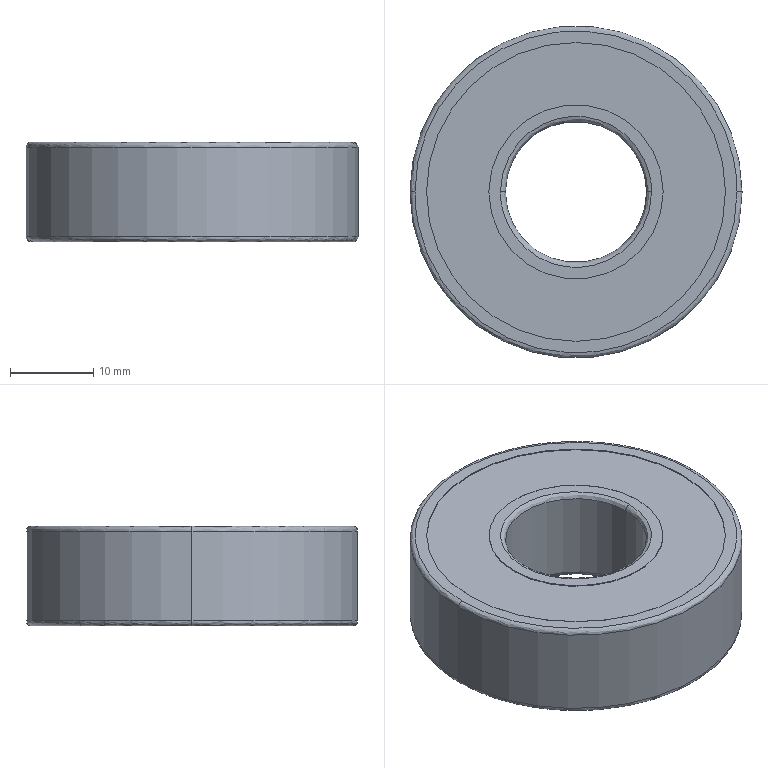Part | SolidWorks | features BaseBody 1 | 1 solid | 26 faces | box 40 x 40 x 12 mm | volume 12195 mm3 | cylinder 12 | spline 8 | plane 6 | commonest cylinder face diameters 21 x4 36 x4 17 x2 40 x2
STEP:
#1=CARTESIAN_POINT('',(-19.4,0.,-12.));
#2=VERTEX_POINT('',#1);
#3=CARTESIAN_POINT('',(19.4,0.,-12.));
#4=VERTEX_POINT('',#3);
#5=CARTESIAN_POINT('',(-19.4,0.,-12.));
#6=CARTESIAN_POINT('',(-19.4,-38.8,-12.));
#7=CARTESIAN_POINT('',(19.4,-38.8,-12.));
#8=CARTESIAN_POINT('',(19.4,0.,-12.));
#9=(BOUNDED_CURVE()B_SPLINE_CURVE(3,(#5,#6,#7,#8),.UNSPECIFIED.,.F.,.F.)B_SPLINE_CURVE_WITH_KNOTS((4,4),(0.,0.5),.UNSPECIFIED.)CURVE()GEOMETRIC_REPRESENTATION_ITEM()RATIONAL_B_SPLINE_CURVE((1.,0.3333,0.3333,1.))REPRESENTATION_ITEM(''));
#10=EDGE_CURVE('',#2,#4,#9,.T.);
#11=ORIENTED_EDGE('',*,*,#10,.T.);
#12=CARTESIAN_POINT('',(20.,0.,-11.4));
#13=VERTEX_POINT('',#12);
#14=CARTESIAN_POINT('',(19.4,0.,-11.4));
#15=DIRECTION('',(0.,-1.,0.));
#16=DIRECTION('',(1.,0.,0.));
#17=AXIS2_PLACEMENT_3D('',#14,#15,#16);
#18=CIRCLE('',#17,0.6);
#19=EDGE_CURVE('',#4,#13,#18,.T.);
#20=ORIENTED_EDGE('',*,*,#19,.T.);
#21=CARTESIAN_POINT('',(-20.,0.,-11.4));
#22=VERTEX_POINT('',#21);
#23=CARTESIAN_POINT('',(0.,0.,-11.4));
#24=DIRECTION('',(0.,0.,1.));
#25=DIRECTION('',(1.,0.,0.));
#26=AXIS2_PLACEMENT_3D('',#23,#24,#25);
#27=CIRCLE('',#26,20.);
#28=EDGE_CURVE('',#22,#13,#27,.T.);
#29=ORIENTED_EDGE('',*,*,#28,.F.);
#30=CARTESIAN_POINT('',(-19.4,0.,-11.4));
#31=DIRECTION('',(0.,1.,0.));
#32=DIRECTION('',(-1.,0.,0.));
#33=AXIS2_PLACEMENT_3D('',#30,#31,#32);
#34=CIRCLE('',#33,0.6);
#35=EDGE_CURVE('',#2,#22,#34,.T.);
#36=ORIENTED_EDGE('',*,*,#35,.F.);
#37=EDGE_LOOP('',(#11,#20,#29,#36));
#38=FACE_OUTER_BOUND('',#37,.T.);
#39=CARTESIAN_POINT('',(19.4,0.,-12.));
#40=CARTESIAN_POINT('',(19.4,-38.8,-12.));
#41=CARTESIAN_POINT('',(-19.4,-38.8,-12.));
#42=CARTESIAN_POINT('',(-19.4,0.,-12.));
#43=CARTESIAN_POINT('',(19.751,0.,-12.));
#44=CARTESIAN_POINT('',(19.751,-39.503,-12.));
#45=CARTESIAN_POINT('',(-19.751,-39.503,-12.));
#46=CARTESIAN_POINT('',(-19.751,0.,-12.));
#47=CARTESIAN_POINT('',(20.,0.,-11.751));
#48=CARTESIAN_POINT('',(20.,-40.,-11.751));
#49=CARTESIAN_POINT('',(-20.,-40.,-11.751));
#50=CARTESIAN_POINT('',(-20.,0.,-11.751));
#51=CARTESIAN_POINT('',(20.,0.,-11.4));
#52=CARTESIAN_POINT('',(20.,-40.,-11.4));
#53=CARTESIAN_POINT('',(-20.,-40.,-11.4));
#54=CARTESIAN_POINT('',(-20.,0.,-11.4));
#55=(BOUNDED_SURFACE()B_SPLINE_SURFACE(3,3,((#39,#40,#41,#42),(#43,#44,#45,#46),(#47,#48,#49,#50),(#51,#52,#53,#54)),.UNSPECIFIED.,.F.,.F.,.F.)B_SPLINE_SURFACE_WITH_KNOTS((4,4),(4,4),(0.,1.),(0.,1.),.UNSPECIFIED.)GEOMETRIC_REPRESENTATION_ITEM()RATIONAL_B_SPLINE_SURFACE(((1.,0.3333,0.3333,1.),(0.8047,0.2682,0.2682,0.8047),(0.8047,0.2682,0.2682,0.8047),(1.,0.3333,0.3333,1.)))REPRESENTATION_ITEM('')SURFACE());
#56=ADVANCED_FACE('',(#38),#55,.T.);
#57=CARTESIAN_POINT('',(20.,0.,-0.6));
#58=VERTEX_POINT('',#57);
#59=CARTESIAN_POINT('',(-20.,0.,-0.6));
#60=VERTEX_POINT('',#59);
#61=CARTESIAN_POINT('',(0.,0.,-0.6));
#62=DIRECTION('',(0.,0.,-1.));
#63=DIRECTION('',(1.,0.,0.));
#64=AXIS2_PLACEMENT_3D('',#61,#62,#63);
#65=CIRCLE('',#64,20.);
#66=EDGE_CURVE('',#58,#60,#65,.T.);
#67=ORIENTED_EDGE('',*,*,#66,.F.);
#68=CARTESIAN_POINT('',(19.4,0.,0.));
#69=VERTEX_POINT('',#68);
#70=CARTESIAN_POINT('',(19.4,0.,-0.6));
#71=DIRECTION('',(0.,-1.,0.));
#72=DIRECTION('',(1.,0.,0.));
#73=AXIS2_PLACEMENT_3D('',#70,#71,#72);
#74=CIRCLE('',#73,0.6);
#75=EDGE_CURVE('',#58,#69,#74,.T.);
#76=ORIENTED_EDGE('',*,*,#75,.T.);
#77=CARTESIAN_POINT('',(-19.4,0.,0.));
#78=VERTEX_POINT('',#77);
#79=CARTESIAN_POINT('',(19.4,0.,0.));
#80=CARTESIAN_POINT('',(19.4,-38.8,0.));
#81=CARTESIAN_POINT('',(-19.4,-38.8,0.));
#82=CARTESIAN_POINT('',(-19.4,0.,0.));
#83=(BOUNDED_CURVE()B_SPLINE_CURVE(3,(#79,#80,#81,#82),.UNSPECIFIED.,.F.,.F.)B_SPLINE_CURVE_WITH_KNOTS((4,4),(0.5,1.),.UNSPECIFIED.)CURVE()GEOMETRIC_REPRESENTATION_ITEM()RATIONAL_B_SPLINE_CURVE((1.,0.3333,0.3333,1.))REPRESENTATION_ITEM(''));
#84=EDGE_CURVE('',#69,#78,#83,.T.);
#85=ORIENTED_EDGE('',*,*,#84,.T.);
#86=CARTESIAN_POINT('',(-19.4,0.,-0.6));
#87=DIRECTION('',(0.,1.,0.));
#88=DIRECTION('',(-1.,0.,0.));
#89=AXIS2_PLACEMENT_3D('',#86,#87,#88);
#90=CIRCLE('',#89,0.6);
#91=EDGE_CURVE('',#60,#78,#90,.T.);
#92=ORIENTED_EDGE('',*,*,#91,.F.);
#93=EDGE_LOOP('',(#67,#76,#85,#92));
#94=FACE_OUTER_BOUND('',#93,.T.);
#95=CARTESIAN_POINT('',(20.,0.,-0.6));
#96=CARTESIAN_POINT('',(20.,-40.,-0.6));
#97=CARTESIAN_POINT('',(-20.,-40.,-0.6));
#98=CARTESIAN_POINT('',(-20.,0.,-0.6));
#99=CARTESIAN_POINT('',(20.,0.,-0.2485));
#100=CARTESIAN_POINT('',(20.,-40.,-0.2485));
#101=CARTESIAN_POINT('',(-20.,-40.,-0.2485));
#102=CARTESIAN_POINT('',(-20.,0.,-0.2485));
#103=CARTESIAN_POINT('',(19.751,0.,0.));
#104=CARTESIAN_POINT('',(19.751,-39.503,0.));
#105=CARTESIAN_POINT('',(-19.751,-39.503,0.));
#106=CARTESIAN_POINT('',(-19.751,0.,0.));
#107=CARTESIAN_POINT('',(19.4,0.,0.));
#108=CARTESIAN_POINT('',(19.4,-38.8,0.));
#109=CARTESIAN_POINT('',(-19.4,-38.8,0.));
#110=CARTESIAN_POINT('',(-19.4,0.,0.));
#111=(BOUNDED_SURFACE()B_SPLINE_SURFACE(3,3,((#95,#96,#97,#98),(#99,#100,#101,#102),(#103,#104,#105,#106),(#107,#108,#109,#110)),.UNSPECIFIED.,.F.,.F.,.F.)B_SPLINE_SURFACE_WITH_KNOTS((4,4),(4,4),(0.,1.),(0.,1.),.UNSPECIFIED.)GEOMETRIC_REPRESENTATION_ITEM()RATIONAL_B_SPLINE_SURFACE(((1.,0.3333,0.3333,1.),(0.8047,0.2682,0.2682,0.8047),(0.8047,0.2682,0.2682,0.8047),(1.,0.3333,0.3333,1.)))REPRESENTATION_ITEM('')SURFACE());
#112=ADVANCED_FACE('',(#94),#111,.T.);
#113=CARTESIAN_POINT('',(-8.5,0.,-11.4));
#114=VERTEX_POINT('',#113);
#115=CARTESIAN_POINT('',(8.5,0.,-11.4));
#116=VERTEX_POINT('',#115);
#117=CARTESIAN_POINT('',(0.,0.,-11.4));
#118=DIRECTION('',(0.,0.,1.));
#119=DIRECTION('',(-1.,0.,0.));
#120=AXIS2_PLACEMENT_3D('',#117,#118,#119);
#121=CIRCLE('',#120,8.5);
#122=EDGE_CURVE('',#114,#116,#121,.T.);
#123=ORIENTED_EDGE('',*,*,#122,.T.);
#124=CARTESIAN_POINT('',(9.1,0.,-12.));
#125=VERTEX_POINT('',#124);
#126=CARTESIAN_POINT('',(9.1,0.,-11.4));
#127=DIRECTION('',(0.,-1.,0.));
#128=DIRECTION('',(1.,0.,0.));
#129=AXIS2_PLACEMENT_3D('',#126,#127,#128);
#130=CIRCLE('',#129,0.6);
#131=EDGE_CURVE('',#116,#125,#130,.T.);
#132=ORIENTED_EDGE('',*,*,#131,.T.);
#133=CARTESIAN_POINT('',(-9.1,0.,-12.));
#134=VERTEX_POINT('',#133);
#135=CARTESIAN_POINT('',(-9.1,0.,-12.));
#136=CARTESIAN_POINT('',(-9.1,-0.2782,-12.));
#137=CARTESIAN_POINT('',(-9.081,-0.6939,-12.));
#138=CARTESIAN_POINT('',(-9.026,-1.176,-12.));
#139=CARTESIAN_POINT('',(-8.99,-1.416,-12.));
#140=CARTESIAN_POINT('',(-8.972,-1.519,-12.));
#141=CARTESIAN_POINT('',(-8.961,-1.587,-12.));
#142=CARTESIAN_POINT('',(-8.955,-1.62,-12.));
#143=CARTESIAN_POINT('',(-8.894,-1.946,-12.));
#144=CARTESIAN_POINT('',(-8.793,-2.375,-12.));
#145=CARTESIAN_POINT('',(-8.639,-2.866,-12.));
#146=CARTESIAN_POINT('',(-8.553,-3.109,-12.));
#147=CARTESIAN_POINT('',(-8.514,-3.212,-12.));
#148=CARTESIAN_POINT('',(-8.488,-3.281,-12.));
#149=CARTESIAN_POINT('',(-8.475,-3.314,-12.));
#150=CARTESIAN_POINT('',(-8.348,-3.635,-12.));
#151=CARTESIAN_POINT('',(-8.158,-4.054,-12.));
#152=CARTESIAN_POINT('',(-7.899,-4.523,-12.));
#153=CARTESIAN_POINT('',(-7.781,-4.72,-12.));
#154=CARTESIAN_POINT('',(-7.7,-4.85,-12.));
#155=CARTESIAN_POINT('',(-7.66,-4.914,-12.));
#156=CARTESIAN_POINT('',(-7.273,-5.505,-12.));
#157=CARTESIAN_POINT('',(-6.879,-5.991,-12.));
#158=CARTESIAN_POINT('',(-6.213,-6.657,-12.));
#159=CARTESIAN_POINT('',(-5.864,-6.971,-12.));
#160=CARTESIAN_POINT('',(-5.431,-7.305,-12.));
#161=CARTESIAN_POINT('',(-5.239,-7.441,-12.));
#162=CARTESIAN_POINT('',(-5.11,-7.53,-12.));
#163=CARTESIAN_POINT('',(-5.044,-7.575,-12.));
#164=CARTESIAN_POINT('',(-4.722,-7.785,-12.));
#165=CARTESIAN_POINT('',(-4.326,-8.017,-12.));
#166=CARTESIAN_POINT('',(-3.844,-8.251,-12.));
#167=CARTESIAN_POINT('',(-3.598,-8.359,-12.));
#168=CARTESIAN_POINT('',(-3.492,-8.403,-12.));
#169=CARTESIAN_POINT('',(-3.421,-8.433,-12.));
#170=CARTESIAN_POINT('',(-3.384,-8.448,-12.));
#171=CARTESIAN_POINT('',(-3.075,-8.57,-12.));
#172=CARTESIAN_POINT('',(-2.658,-8.712,-12.));
#173=CARTESIAN_POINT('',(-2.16,-8.842,-12.));
#174=CARTESIAN_POINT('',(-1.909,-8.898,-12.));
#175=CARTESIAN_POINT('',(-1.801,-8.92,-12.));
#176=CARTESIAN_POINT('',(-1.728,-8.934,-12.));
#177=CARTESIAN_POINT('',(-1.69,-8.942,-12.));
#178=CARTESIAN_POINT('',(-1.109,-9.049,-12.));
#179=CARTESIAN_POINT('',(-0.5562,-9.1,-12.));
#180=CARTESIAN_POINT('',(0.2781,-9.1,-12.));
#181=CARTESIAN_POINT('',(0.6937,-9.081,-12.));
#182=CARTESIAN_POINT('',(1.176,-9.026,-12.));
#183=CARTESIAN_POINT('',(1.416,-8.99,-12.));
#184=CARTESIAN_POINT('',(1.519,-8.972,-12.));
#185=CARTESIAN_POINT('',(1.587,-8.961,-12.));
#186=CARTESIAN_POINT('',(1.62,-8.955,-12.));
#187=CARTESIAN_POINT('',(1.946,-8.894,-12.));
#188=CARTESIAN_POINT('',(2.375,-8.793,-12.));
#189=CARTESIAN_POINT('',(2.866,-8.639,-12.));
#190=CARTESIAN_POINT('',(3.109,-8.553,-12.));
#191=CARTESIAN_POINT('',(3.212,-8.514,-12.));
#192=CARTESIAN_POINT('',(3.281,-8.488,-12.));
#193=CARTESIAN_POINT('',(3.314,-8.475,-12.));
#194=CARTESIAN_POINT('',(3.635,-8.348,-12.));
#195=CARTESIAN_POINT('',(4.054,-8.158,-12.));
#196=CARTESIAN_POINT('',(4.523,-7.899,-12.));
#197=CARTESIAN_POINT('',(4.72,-7.781,-12.));
#198=CARTESIAN_POINT('',(4.85,-7.7,-12.));
#199=CARTESIAN_POINT('',(4.914,-7.66,-12.));
#200=CARTESIAN_POINT('',(5.505,-7.273,-12.));
#201=CARTESIAN_POINT('',(5.991,-6.879,-12.));
#202=CARTESIAN_POINT('',(6.657,-6.213,-12.));
#203=CARTESIAN_POINT('',(6.971,-5.864,-12.));
#204=CARTESIAN_POINT('',(7.305,-5.431,-12.));
#205=CARTESIAN_POINT('',(7.441,-5.239,-12.));
#206=CARTESIAN_POINT('',(7.53,-5.11,-12.));
#207=CARTESIAN_POINT('',(7.575,-5.044,-12.));
#208=CARTESIAN_POINT('',(7.785,-4.722,-12.));
#209=CARTESIAN_POINT('',(8.017,-4.326,-12.));
#210=CARTESIAN_POINT('',(8.251,-3.844,-12.));
#211=CARTESIAN_POINT('',(8.359,-3.598,-12.));
#212=CARTESIAN_POINT('',(8.403,-3.492,-12.));
#213=CARTESIAN_POINT('',(8.433,-3.421,-12.));
#214=CARTESIAN_POINT('',(8.448,-3.384,-12.));
#215=CARTESIAN_POINT('',(8.57,-3.075,-12.));
#216=CARTESIAN_POINT('',(8.712,-2.658,-12.));
#217=CARTESIAN_POINT('',(8.842,-2.16,-12.));
#218=CARTESIAN_POINT('',(8.898,-1.909,-12.));
#219=CARTESIAN_POINT('',(8.92,-1.801,-12.));
#220=CARTESIAN_POINT('',(8.934,-1.728,-12.));
#221=CARTESIAN_POINT('',(8.942,-1.69,-12.));
#222=CARTESIAN_POINT('',(9.049,-1.109,-12.));
#223=CARTESIAN_POINT('',(9.1,-0.5562,-12.));
#224=CARTESIAN_POINT('',(9.1,0.,-12.));
#225=B_SPLINE_CURVE_WITH_KNOTS('',3,(#135,#136,#137,#138,#139,#140,#141,#142,#143,#144,#145,#146,#147,#148,#149,#150,#151,#152,#153,#154,#155,#156,#157,#158,#159,#160,#161,#162,#163,#164,#165,#166,#167,#168,#169,#170,#171,#172,#173,#174,#175,#176,#177,#178,#179,#180,#181,#182,#183,#184,#185,#186,#187,#188,#189,#190,#191,#192,#193,#194,#195,#196,#197,#198,#199,#200,#201,#202,#203,#204,#205,#206,#207,#208,#209,#210,#211,#212,#213,#214,#215,#216,#217,#218,#219,#220,#221,#222,#223,#224),.UNSPECIFIED.,.F.,.F.,(4,1,1,1,2,2,1,1,1,2,2,1,1,2,2,2,1,1,2,2,1,1,1,2,2,1,1,1,2,2,2,1,1,1,2,2,1,1,1,2,2,1,1,2,2,2,1,1,2,2,1,1,1,2,2,1,1,1,2,2,4),(0.,0.01562,0.02344,0.02734,0.0293,0.03125,0.04687,0.05469,0.05859,0.06055,0.0625,0.07812,0.08594,0.08984,0.09375,0.125,0.1406,0.1484,0.1523,0.1562,0.1719,0.1797,0.1836,0.1855,0.1875,0.2031,0.2109,0.2148,0.2168,0.2187,0.25,0.2656,0.2734,0.2773,0.2793,0.2812,0.2969,0.3047,0.3086,0.3105,0.3125,0.3281,0.3359,0.3398,0.3437,0.375,0.3906,0.3984,0.4023,0.4062,0.4219,0.4297,0.4336,0.4355,0.4375,0.4531,0.4609,0.4648,0.4668,0.4687,0.5),.UNSPECIFIED.);
#226=EDGE_CURVE('',#134,#125,#225,.T.);
#227=ORIENTED_EDGE('',*,*,#226,.F.);
#228=CARTESIAN_POINT('',(-9.1,0.,-11.4));
#229=DIRECTION('',(0.,1.,0.));
#230=DIRECTION('',(-1.,0.,0.));
#231=AXIS2_PLACEMENT_3D('',#228,#229,#230);
#232=CIRCLE('',#231,0.6);
#233=EDGE_CURVE('',#114,#134,#232,.T.);
#234=ORIENTED_EDGE('',*,*,#233,.F.);
#235=EDGE_LOOP('',(#123,#132,#227,#234));
#236=FACE_OUTER_BOUND('',#235,.T.);
#237=CARTESIAN_POINT('',(8.5,0.,-11.4));
#238=CARTESIAN_POINT('',(8.5,-17.,-11.4));
#239=CARTESIAN_POINT('',(-8.5,-17.,-11.4));
#240=CARTESIAN_POINT('',(-8.5,0.,-11.4));
#241=CARTESIAN_POINT('',(8.5,0.,-11.751));
#242=CARTESIAN_POINT('',(8.5,-17.,-11.751));
#243=CARTESIAN_POINT('',(-8.5,-17.,-11.751));
#244=CARTESIAN_POINT('',(-8.5,0.,-11.751));
#245=CARTESIAN_POINT('',(8.749,0.,-12.));
#246=CARTESIAN_POINT('',(8.749,-17.497,-12.));
#247=CARTESIAN_POINT('',(-8.749,-17.497,-12.));
#248=CARTESIAN_POINT('',(-8.749,0.,-12.));
#249=CARTESIAN_POINT('',(9.1,0.,-12.));
#250=CARTESIAN_POINT('',(9.1,-18.2,-12.));
#251=CARTESIAN_POINT('',(-9.1,-18.2,-12.));
#252=CARTESIAN_POINT('',(-9.1,0.,-12.));
#253=(BOUNDED_SURFACE()B_SPLINE_SURFACE(3,3,((#237,#238,#239,#240),(#241,#242,#243,#244),(#245,#246,#247,#248),(#249,#250,#251,#252)),.UNSPECIFIED.,.F.,.F.,.F.)B_SPLINE_SURFACE_WITH_KNOTS((4,4),(4,4),(0.,1.),(0.,1.),.UNSPECIFIED.)GEOMETRIC_REPRESENTATION_ITEM()RATIONAL_B_SPLINE_SURFACE(((1.,0.3333,0.3333,1.),(0.8047,0.2682,0.2682,0.8047),(0.8047,0.2682,0.2682,0.8047),(1.,0.3333,0.3333,1.)))REPRESENTATION_ITEM('')SURFACE());
#254=ADVANCED_FACE('',(#236),#253,.T.);
#255=CARTESIAN_POINT('',(9.1,0.,0.));
#256=VERTEX_POINT('',#255);
#257=CARTESIAN_POINT('',(-9.1,0.,0.));
#258=VERTEX_POINT('',#257);
#259=CARTESIAN_POINT('',(9.1,0.,0.));
#260=CARTESIAN_POINT('',(9.1,-0.2781,0.));
#261=CARTESIAN_POINT('',(9.081,-0.6937,0.));
#262=CARTESIAN_POINT('',(9.026,-1.176,0.));
#263=CARTESIAN_POINT('',(8.99,-1.416,0.));
#264=CARTESIAN_POINT('',(8.972,-1.519,0.));
#265=CARTESIAN_POINT('',(8.961,-1.587,0.));
#266=CARTESIAN_POINT('',(8.955,-1.62,0.));
#267=CARTESIAN_POINT('',(8.894,-1.946,0.));
#268=CARTESIAN_POINT('',(8.793,-2.375,0.));
#269=CARTESIAN_POINT('',(8.639,-2.866,0.));
#270=CARTESIAN_POINT('',(8.553,-3.109,0.));
#271=CARTESIAN_POINT('',(8.514,-3.212,0.));
#272=CARTESIAN_POINT('',(8.488,-3.281,0.));
#273=CARTESIAN_POINT('',(8.475,-3.314,0.));
#274=CARTESIAN_POINT('',(8.348,-3.635,0.));
#275=CARTESIAN_POINT('',(8.158,-4.054,0.));
#276=CARTESIAN_POINT('',(7.899,-4.523,0.));
#277=CARTESIAN_POINT('',(7.781,-4.72,0.));
#278=CARTESIAN_POINT('',(7.7,-4.85,0.));
#279=CARTESIAN_POINT('',(7.66,-4.914,0.));
#280=CARTESIAN_POINT('',(7.273,-5.505,0.));
#281=CARTESIAN_POINT('',(6.879,-5.991,0.));
#282=CARTESIAN_POINT('',(6.213,-6.657,0.));
#283=CARTESIAN_POINT('',(5.864,-6.971,0.));
#284=CARTESIAN_POINT('',(5.431,-7.305,0.));
#285=CARTESIAN_POINT('',(5.239,-7.441,0.));
#286=CARTESIAN_POINT('',(5.11,-7.53,0.));
#287=CARTESIAN_POINT('',(5.044,-7.575,0.));
#288=CARTESIAN_POINT('',(4.722,-7.785,0.));
#289=CARTESIAN_POINT('',(4.326,-8.017,0.));
#290=CARTESIAN_POINT('',(3.844,-8.251,0.));
#291=CARTESIAN_POINT('',(3.598,-8.359,0.));
#292=CARTESIAN_POINT('',(3.492,-8.403,0.));
#293=CARTESIAN_POINT('',(3.421,-8.433,0.));
#294=CARTESIAN_POINT('',(3.384,-8.448,0.));
#295=CARTESIAN_POINT('',(3.075,-8.57,0.));
#296=CARTESIAN_POINT('',(2.658,-8.712,0.));
#297=CARTESIAN_POINT('',(2.16,-8.842,0.));
#298=CARTESIAN_POINT('',(1.909,-8.898,0.));
#299=CARTESIAN_POINT('',(1.801,-8.92,0.));
#300=CARTESIAN_POINT('',(1.728,-8.934,0.));
#301=CARTESIAN_POINT('',(1.69,-8.942,0.));
#302=CARTESIAN_POINT('',(1.109,-9.049,0.));
#303=CARTESIAN_POINT('',(0.5562,-9.1,0.));
#304=CARTESIAN_POINT('',(-0.2781,-9.1,0.));
#305=CARTESIAN_POINT('',(-0.6937,-9.081,0.));
#306=CARTESIAN_POINT('',(-1.176,-9.026,0.));
#307=CARTESIAN_POINT('',(-1.416,-8.99,0.));
#308=CARTESIAN_POINT('',(-1.519,-8.972,0.));
#309=CARTESIAN_POINT('',(-1.587,-8.961,0.));
#310=CARTESIAN_POINT('',(-1.62,-8.955,0.));
#311=CARTESIAN_POINT('',(-1.946,-8.894,0.));
#312=CARTESIAN_POINT('',(-2.375,-8.793,0.));
#313=CARTESIAN_POINT('',(-2.866,-8.639,0.));
#314=CARTESIAN_POINT('',(-3.109,-8.553,0.));
#315=CARTESIAN_POINT('',(-3.212,-8.514,0.));
#316=CARTESIAN_POINT('',(-3.281,-8.488,0.));
#317=CARTESIAN_POINT('',(-3.314,-8.475,0.));
#318=CARTESIAN_POINT('',(-3.635,-8.348,0.));
#319=CARTESIAN_POINT('',(-4.054,-8.158,0.));
#320=CARTESIAN_POINT('',(-4.523,-7.899,0.));
#321=CARTESIAN_POINT('',(-4.72,-7.781,0.));
#322=CARTESIAN_POINT('',(-4.85,-7.7,0.));
#323=CARTESIAN_POINT('',(-4.914,-7.66,0.));
#324=CARTESIAN_POINT('',(-5.505,-7.273,0.));
#325=CARTESIAN_POINT('',(-5.991,-6.879,0.));
#326=CARTESIAN_POINT('',(-6.657,-6.213,0.));
#327=CARTESIAN_POINT('',(-6.971,-5.864,0.));
#328=CARTESIAN_POINT('',(-7.305,-5.431,0.));
#329=CARTESIAN_POINT('',(-7.441,-5.239,0.));
#330=CARTESIAN_POINT('',(-7.53,-5.11,0.));
#331=CARTESIAN_POINT('',(-7.575,-5.044,0.));
#332=CARTESIAN_POINT('',(-7.785,-4.722,0.));
#333=CARTESIAN_POINT('',(-8.017,-4.326,0.));
#334=CARTESIAN_POINT('',(-8.251,-3.844,0.));
#335=CARTESIAN_POINT('',(-8.359,-3.598,0.));
#336=CARTESIAN_POINT('',(-8.403,-3.492,0.));
#337=CARTESIAN_POINT('',(-8.433,-3.421,0.));
#338=CARTESIAN_POINT('',(-8.448,-3.384,0.));
#339=CARTESIAN_POINT('',(-8.57,-3.075,0.));
#340=CARTESIAN_POINT('',(-8.712,-2.658,0.));
#341=CARTESIAN_POINT('',(-8.842,-2.16,0.));
#342=CARTESIAN_POINT('',(-8.898,-1.909,0.));
#343=CARTESIAN_POINT('',(-8.92,-1.801,0.));
#344=CARTESIAN_POINT('',(-8.934,-1.728,0.));
#345=CARTESIAN_POINT('',(-8.942,-1.69,0.));
#346=CARTESIAN_POINT('',(-9.049,-1.109,0.));
#347=CARTESIAN_POINT('',(-9.1,-0.5568,0.));
#348=CARTESIAN_POINT('',(-9.1,0.,0.));
#349=B_SPLINE_CURVE_WITH_KNOTS('',3,(#259,#260,#261,#262,#263,#264,#265,#266,#267,#268,#269,#270,#271,#272,#273,#274,#275,#276,#277,#278,#279,#280,#281,#282,#283,#284,#285,#286,#287,#288,#289,#290,#291,#292,#293,#294,#295,#296,#297,#298,#299,#300,#301,#302,#303,#304,#305,#306,#307,#308,#309,#310,#311,#312,#313,#314,#315,#316,#317,#318,#319,#320,#321,#322,#323,#324,#325,#326,#327,#328,#329,#330,#331,#332,#333,#334,#335,#336,#337,#338,#339,#340,#341,#342,#343,#344,#345,#346,#347,#348),.UNSPECIFIED.,.F.,.F.,(4,1,1,1,2,2,1,1,1,2,2,1,1,2,2,2,1,1,2,2,1,1,1,2,2,1,1,1,2,2,2,1,1,1,2,2,1,1,1,2,2,1,1,2,2,2,1,1,2,2,1,1,1,2,2,1,1,1,2,2,4),(0.5,0.5156,0.5234,0.5273,0.5293,0.5312,0.5469,0.5547,0.5586,0.5605,0.5625,0.5781,0.5859,0.5898,0.5937,0.625,0.6406,0.6484,0.6523,0.6562,0.6719,0.6797,0.6836,0.6855,0.6875,0.7031,0.7109,0.7148,0.7168,0.7188,0.75,0.7656,0.7734,0.7773,0.7793,0.7812,0.7969,0.8047,0.8086,0.8105,0.8125,0.8281,0.8359,0.8398,0.8437,0.875,0.8906,0.8984,0.9023,0.9062,0.9219,0.9297,0.9336,0.9355,0.9375,0.9531,0.9609,0.9648,0.9668,0.9687,1.),.UNSPECIFIED.);
#350=EDGE_CURVE('',#256,#258,#349,.T.);
#351=ORIENTED_EDGE('',*,*,#350,.F.);
#352=CARTESIAN_POINT('',(8.5,0.,-0.6));
#353=VERTEX_POINT('',#352);
#354=CARTESIAN_POINT('',(9.1,0.,-0.6));
#355=DIRECTION('',(0.,-1.,0.));
#356=DIRECTION('',(1.,0.,0.));
#357=AXIS2_PLACEMENT_3D('',#354,#355,#356);
#358=CIRCLE('',#357,0.6);
#359=EDGE_CURVE('',#256,#353,#358,.T.);
#360=ORIENTED_EDGE('',*,*,#359,.T.);
#361=CARTESIAN_POINT('',(-8.5,0.,-0.6));
#362=VERTEX_POINT('',#361);
#363=CARTESIAN_POINT('',(0.,0.,-0.6));
#364=DIRECTION('',(0.,0.,-1.));
#365=DIRECTION('',(-1.,0.,0.));
#366=AXIS2_PLACEMENT_3D('',#363,#364,#365);
#367=CIRCLE('',#366,8.5);
#368=EDGE_CURVE('',#353,#362,#367,.T.);
#369=ORIENTED_EDGE('',*,*,#368,.T.);
#370=CARTESIAN_POINT('',(-9.1,0.,-0.6));
#371=DIRECTION('',(0.,1.,0.));
#372=DIRECTION('',(-1.,0.,0.));
#373=AXIS2_PLACEMENT_3D('',#370,#371,#372);
#374=CIRCLE('',#373,0.6);
#375=EDGE_CURVE('',#258,#362,#374,.T.);
#376=ORIENTED_EDGE('',*,*,#375,.F.);
#377=EDGE_LOOP('',(#351,#360,#369,#376));
#378=FACE_OUTER_BOUND('',#377,.T.);
#379=CARTESIAN_POINT('',(9.1,0.,0.));
#380=CARTESIAN_POINT('',(9.1,-18.2,0.));
#381=CARTESIAN_POINT('',(-9.1,-18.2,0.));
#382=CARTESIAN_POINT('',(-9.1,0.,0.));
#383=CARTESIAN_POINT('',(8.749,0.,0.));
#384=CARTESIAN_POINT('',(8.749,-17.497,0.));
#385=CARTESIAN_POINT('',(-8.749,-17.497,0.));
#386=CARTESIAN_POINT('',(-8.749,0.,0.));
#387=CARTESIAN_POINT('',(8.5,0.,-0.2485));
#388=CARTESIAN_POINT('',(8.5,-17.,-0.2485));
#389=CARTESIAN_POINT('',(-8.5,-17.,-0.2485));
#390=CARTESIAN_POINT('',(-8.5,0.,-0.2485));
#391=CARTESIAN_POINT('',(8.5,0.,-0.6));
#392=CARTESIAN_POINT('',(8.5,-17.,-0.6));
#393=CARTESIAN_POINT('',(-8.5,-17.,-0.6));
#394=CARTESIAN_POINT('',(-8.5,0.,-0.6));
#395=(BOUNDED_SURFACE()B_SPLINE_SURFACE(3,3,((#379,#380,#381,#382),(#383,#384,#385,#386),(#387,#388,#389,#390),(#391,#392,#393,#394)),.UNSPECIFIED.,.F.,.F.,.F.)B_SPLINE_SURFACE_WITH_KNOTS((4,4),(4,4),(0.,1.),(0.,1.),.UNSPECIFIED.)GEOMETRIC_REPRESENTATION_ITEM()RATIONAL_B_SPLINE_SURFACE(((1.,0.3333,0.3333,1.),(0.8047,0.2682,0.2682,0.8047),(0.8047,0.2682,0.2682,0.8047),(1.,0.3333,0.3333,1.)))REPRESENTATION_ITEM('')SURFACE());
#396=ADVANCED_FACE('',(#378),#395,.T.);
#397=CARTESIAN_POINT('',(0.,0.,-11.4));
#398=DIRECTION('',(0.,0.,1.));
#399=DIRECTION('',(1.,0.,0.));
#400=AXIS2_PLACEMENT_3D('',#397,#398,#399);
#401=CIRCLE('',#400,20.);
#402=EDGE_CURVE('',#13,#22,#401,.T.);
#403=ORIENTED_EDGE('',*,*,#402,.T.);
#404=CARTESIAN_POINT('',(-20.,0.,-12.));
#405=DIRECTION('',(0.,0.,1.));
#406=VECTOR('',#405,1000.);
#407=LINE('',#404,#406);
#408=EDGE_CURVE('',#22,#60,#407,.T.);
#409=ORIENTED_EDGE('',*,*,#408,.T.);
#410=CARTESIAN_POINT('',(0.,0.,-0.6));
#411=DIRECTION('',(0.,0.,-1.));
#412=DIRECTION('',(1.,0.,0.));
#413=AXIS2_PLACEMENT_3D('',#410,#411,#412);
#414=CIRCLE('',#413,20.);
#415=EDGE_CURVE('',#60,#58,#414,.T.);
#416=ORIENTED_EDGE('',*,*,#415,.T.);
#417=CARTESIAN_POINT('',(20.,0.,-12.));
#418=DIRECTION('',(0.,0.,1.));
#419=VECTOR('',#418,1000.);
#420=LINE('',#417,#419);
#421=EDGE_CURVE('',#13,#58,#420,.T.);
#422=ORIENTED_EDGE('',*,*,#421,.F.);
#423=EDGE_LOOP('',(#403,#409,#416,#422));
#424=FACE_OUTER_BOUND('',#423,.T.);
#425=CARTESIAN_POINT('',(0.,0.,-12.));
#426=DIRECTION('',(0.,0.,1.));
#427=DIRECTION('',(1.,0.,0.));
#428=AXIS2_PLACEMENT_3D('',#425,#426,#427);
#429=CYLINDRICAL_SURFACE('',#428,20.);
#430=ADVANCED_FACE('',(#424),#429,.T.);
#431=CARTESIAN_POINT('',(-18.,0.,-12.));
#432=VERTEX_POINT('',#431);
#433=CARTESIAN_POINT('',(18.,0.,-12.));
#434=VERTEX_POINT('',#433);
#435=CARTESIAN_POINT('',(0.,0.,-12.));
#436=DIRECTION('',(0.,0.,1.));
#437=DIRECTION('',(1.,0.,0.));
#438=AXIS2_PLACEMENT_3D('',#435,#436,#437);
#439=CIRCLE('',#438,18.);
#440=EDGE_CURVE('',#432,#434,#439,.T.);
#441=ORIENTED_EDGE('',*,*,#440,.F.);
#442=CARTESIAN_POINT('',(-18.,0.,-11.9));
#443=VERTEX_POINT('',#442);
#444=CARTESIAN_POINT('',(-18.,0.,-12.));
#445=DIRECTION('',(0.,0.,1.));
#446=VECTOR('',#445,1000.);
#447=LINE('',#444,#446);
#448=EDGE_CURVE('',#432,#443,#447,.T.);
#449=ORIENTED_EDGE('',*,*,#448,.T.);
#450=CARTESIAN_POINT('',(18.,0.,-11.9));
#451=VERTEX_POINT('',#450);
#452=CARTESIAN_POINT('',(0.,0.,-11.9));
#453=DIRECTION('',(0.,0.,-1.));
#454=DIRECTION('',(1.,0.,0.));
#455=AXIS2_PLACEMENT_3D('',#452,#453,#454);
#456=CIRCLE('',#455,18.);
#457=EDGE_CURVE('',#451,#443,#456,.T.);
#458=ORIENTED_EDGE('',*,*,#457,.F.);
#459=CARTESIAN_POINT('',(18.,0.,-12.));
#460=DIRECTION('',(0.,0.,1.));
#461=VECTOR('',#460,1000.);
#462=LINE('',#459,#461);
#463=EDGE_CURVE('',#434,#451,#462,.T.);
#464=ORIENTED_EDGE('',*,*,#463,.F.);
#465=EDGE_LOOP('',(#441,#449,#458,#464));
#466=FACE_OUTER_BOUND('',#465,.T.);
#467=CARTESIAN_POINT('',(0.,0.,-12.));
#468=DIRECTION('',(0.,0.,1.));
#469=DIRECTION('',(1.,0.,0.));
#470=AXIS2_PLACEMENT_3D('',#467,#468,#469);
#471=CYLINDRICAL_SURFACE('',#470,18.);
#472=ADVANCED_FACE('',(#466),#471,.F.);
#473=CARTESIAN_POINT('',(-18.,0.,-0.1));
#474=VERTEX_POINT('',#473);
#475=CARTESIAN_POINT('',(18.,0.,-0.1));
#476=VERTEX_POINT('',#475);
#477=CARTESIAN_POINT('',(0.,0.,-0.1));
#478=DIRECTION('',(0.,0.,1.));
#479=DIRECTION('',(1.,0.,0.));
#480=AXIS2_PLACEMENT_3D('',#477,#478,#479);
#481=CIRCLE('',#480,18.);
#482=EDGE_CURVE('',#474,#476,#481,.T.);
#483=ORIENTED_EDGE('',*,*,#482,.F.);
#484=CARTESIAN_POINT('',(-18.,0.,0.));
#485=VERTEX_POINT('',#484);
#486=CARTESIAN_POINT('',(-18.,0.,-12.));
#487=DIRECTION('',(0.,0.,1.));
#488=VECTOR('',#487,1000.);
#489=LINE('',#486,#488);
#490=EDGE_CURVE('',#474,#485,#489,.T.);
#491=ORIENTED_EDGE('',*,*,#490,.T.);
#492=CARTESIAN_POINT('',(18.,0.,0.));
#493=VERTEX_POINT('',#492);
#494=CARTESIAN_POINT('',(0.,0.,0.));
#495=DIRECTION('',(0.,0.,-1.));
#496=DIRECTION('',(1.,0.,0.));
#497=AXIS2_PLACEMENT_3D('',#494,#495,#496);
#498=CIRCLE('',#497,18.);
#499=EDGE_CURVE('',#493,#485,#498,.T.);
#500=ORIENTED_EDGE('',*,*,#499,.F.);
#501=CARTESIAN_POINT('',(18.,0.,-12.));
#502=DIRECTION('',(0.,0.,1.));
#503=VECTOR('',#502,1000.);
#504=LINE('',#501,#503);
#505=EDGE_CURVE('',#476,#493,#504,.T.);
#506=ORIENTED_EDGE('',*,*,#505,.F.);
#507=EDGE_LOOP('',(#483,#491,#500,#506));
#508=FACE_OUTER_BOUND('',#507,.T.);
#509=CARTESIAN_POINT('',(0.,0.,-12.));
#510=DIRECTION('',(0.,0.,1.));
#511=DIRECTION('',(1.,0.,0.));
#512=AXIS2_PLACEMENT_3D('',#509,#510,#511);
#513=CYLINDRICAL_SURFACE('',#512,18.);
#514=ADVANCED_FACE('',(#508),#513,.F.);
#515=CARTESIAN_POINT('',(10.5,0.,-12.));
#516=VERTEX_POINT('',#515);
#517=CARTESIAN_POINT('',(-10.5,0.,-12.));
#518=VERTEX_POINT('',#517);
#519=CARTESIAN_POINT('',(0.,0.,-12.));
#520=DIRECTION('',(0.,0.,1.));
#521=DIRECTION('',(1.,0.,0.));
#522=AXIS2_PLACEMENT_3D('',#519,#520,#521);
#523=CIRCLE('',#522,10.5);
#524=EDGE_CURVE('',#516,#518,#523,.T.);
#525=ORIENTED_EDGE('',*,*,#524,.T.);
#526=CARTESIAN_POINT('',(-10.5,0.,-11.9));
#527=VERTEX_POINT('',#526);
#528=CARTESIAN_POINT('',(-10.5,0.,-12.));
#529=DIRECTION('',(0.,0.,1.));
#530=VECTOR('',#529,1000.);
#531=LINE('',#528,#530);
#532=EDGE_CURVE('',#518,#527,#531,.T.);
#533=ORIENTED_EDGE('',*,*,#532,.T.);
#534=CARTESIAN_POINT('',(10.5,0.,-11.9));
#535=VERTEX_POINT('',#534);
#536=CARTESIAN_POINT('',(0.,0.,-11.9));
#537=DIRECTION('',(0.,0.,1.));
#538=DIRECTION('',(1.,0.,0.));
#539=AXIS2_PLACEMENT_3D('',#536,#537,#538);
#540=CIRCLE('',#539,10.5);
#541=EDGE_CURVE('',#535,#527,#540,.T.);
#542=ORIENTED_EDGE('',*,*,#541,.F.);
#543=CARTESIAN_POINT('',(10.5,0.,-12.));
#544=DIRECTION('',(0.,0.,1.));
#545=VECTOR('',#544,1000.);
#546=LINE('',#543,#545);
#547=EDGE_CURVE('',#516,#535,#546,.T.);
#548=ORIENTED_EDGE('',*,*,#547,.F.);
#549=EDGE_LOOP('',(#525,#533,#542,#548));
#550=FACE_OUTER_BOUND('',#549,.T.);
#551=CARTESIAN_POINT('',(0.,0.,-12.));
#552=DIRECTION('',(0.,0.,1.));
#553=DIRECTION('',(1.,0.,0.));
#554=AXIS2_PLACEMENT_3D('',#551,#552,#553);
#555=CYLINDRICAL_SURFACE('',#554,10.5);
#556=ADVANCED_FACE('',(#550),#555,.T.);
#557=CARTESIAN_POINT('',(-10.5,0.,-0.1));
#558=VERTEX_POINT('',#557);
#559=CARTESIAN_POINT('',(10.5,0.,-0.1));
#560=VERTEX_POINT('',#559);
#561=CARTESIAN_POINT('',(0.,0.,-0.1));
#562=DIRECTION('',(0.,0.,-1.));
#563=DIRECTION('',(1.,0.,0.));
#564=AXIS2_PLACEMENT_3D('',#561,#562,#563);
#565=CIRCLE('',#564,10.5);
#566=EDGE_CURVE('',#558,#560,#565,.T.);
#567=ORIENTED_EDGE('',*,*,#566,.F.);
#568=CARTESIAN_POINT('',(-10.5,0.,0.));
#569=VERTEX_POINT('',#568);
#570=CARTESIAN_POINT('',(-10.5,0.,-12.));
#571=DIRECTION('',(0.,0.,1.));
#572=VECTOR('',#571,1000.);
#573=LINE('',#570,#572);
#574=EDGE_CURVE('',#558,#569,#573,.T.);
#575=ORIENTED_EDGE('',*,*,#574,.T.);
#576=CARTESIAN_POINT('',(10.5,0.,0.));
#577=VERTEX_POINT('',#576);
#578=CARTESIAN_POINT('',(0.,0.,0.));
#579=DIRECTION('',(0.,0.,-1.));
#580=DIRECTION('',(1.,0.,0.));
#581=AXIS2_PLACEMENT_3D('',#578,#579,#580);
#582=CIRCLE('',#581,10.5);
#583=EDGE_CURVE('',#569,#577,#582,.T.);
#584=ORIENTED_EDGE('',*,*,#583,.T.);
#585=CARTESIAN_POINT('',(10.5,0.,-12.));
#586=DIRECTION('',(0.,0.,1.));
#587=VECTOR('',#586,1000.);
#588=LINE('',#585,#587);
#589=EDGE_CURVE('',#560,#577,#588,.T.);
#590=ORIENTED_EDGE('',*,*,#589,.F.);
#591=EDGE_LOOP('',(#567,#575,#584,#590));
#592=FACE_OUTER_BOUND('',#591,.T.);
#593=CARTESIAN_POINT('',(0.,0.,-12.));
#594=DIRECTION('',(0.,0.,1.));
#595=DIRECTION('',(1.,0.,0.));
#596=AXIS2_PLACEMENT_3D('',#593,#594,#595);
#597=CYLINDRICAL_SURFACE('',#596,10.5);
#598=ADVANCED_FACE('',(#592),#597,.T.);
#599=ORIENTED_EDGE('',*,*,#122,.F.);
#600=CARTESIAN_POINT('',(-8.5,0.,-12.));
#601=DIRECTION('',(0.,0.,1.));
#602=VECTOR('',#601,1000.);
#603=LINE('',#600,#602);
#604=EDGE_CURVE('',#114,#362,#603,.T.);
#605=ORIENTED_EDGE('',*,*,#604,.T.);
#606=ORIENTED_EDGE('',*,*,#368,.F.);
#607=CARTESIAN_POINT('',(8.5,0.,-12.));
#608=DIRECTION('',(0.,0.,1.));
#609=VECTOR('',#608,1000.);
#610=LINE('',#607,#609);
#611=EDGE_CURVE('',#116,#353,#610,.T.);
#612=ORIENTED_EDGE('',*,*,#611,.F.);
#613=EDGE_LOOP('',(#599,#605,#606,#612));
#614=FACE_OUTER_BOUND('',#613,.T.);
#615=CARTESIAN_POINT('',(0.,0.,-12.));
#616=DIRECTION('',(0.,0.,1.));
#617=DIRECTION('',(1.,0.,0.));
#618=AXIS2_PLACEMENT_3D('',#615,#616,#617);
#619=CYLINDRICAL_SURFACE('',#618,8.5);
#620=ADVANCED_FACE('',(#614),#619,.F.);
#621=ORIENTED_EDGE('',*,*,#408,.F.);
#622=ORIENTED_EDGE('',*,*,#28,.T.);
#623=ORIENTED_EDGE('',*,*,#421,.T.);
#624=ORIENTED_EDGE('',*,*,#66,.T.);
#625=EDGE_LOOP('',(#621,#622,#623,#624));
#626=FACE_OUTER_BOUND('',#625,.T.);
#627=CARTESIAN_POINT('',(0.,0.,-12.));
#628=DIRECTION('',(0.,0.,1.));
#629=DIRECTION('',(1.,0.,0.));
#630=AXIS2_PLACEMENT_3D('',#627,#628,#629);
#631=CYLINDRICAL_SURFACE('',#630,20.);
#632=ADVANCED_FACE('',(#626),#631,.T.);
#633=ORIENTED_EDGE('',*,*,#19,.F.);
#634=CARTESIAN_POINT('',(19.4,0.,-12.));
#635=CARTESIAN_POINT('',(19.4,38.8,-12.));
#636=CARTESIAN_POINT('',(-19.4,38.8,-12.));
#637=CARTESIAN_POINT('',(-19.4,0.,-12.));
#638=(BOUNDED_CURVE()B_SPLINE_CURVE(3,(#634,#635,#636,#637),.UNSPECIFIED.,.F.,.F.)B_SPLINE_CURVE_WITH_KNOTS((4,4),(0.5,1.),.UNSPECIFIED.)CURVE()GEOMETRIC_REPRESENTATION_ITEM()RATIONAL_B_SPLINE_CURVE((1.,0.3333,0.3333,1.))REPRESENTATION_ITEM(''));
#639=EDGE_CURVE('',#4,#2,#638,.T.);
#640=ORIENTED_EDGE('',*,*,#639,.T.);
#641=ORIENTED_EDGE('',*,*,#35,.T.);
#642=ORIENTED_EDGE('',*,*,#402,.F.);
#643=EDGE_LOOP('',(#633,#640,#641,#642));
#644=FACE_OUTER_BOUND('',#643,.T.);
#645=CARTESIAN_POINT('',(-19.4,0.,-12.));
#646=CARTESIAN_POINT('',(-19.4,38.8,-12.));
#647=CARTESIAN_POINT('',(19.4,38.8,-12.));
#648=CARTESIAN_POINT('',(19.4,0.,-12.));
#649=CARTESIAN_POINT('',(-19.751,0.,-12.));
#650=CARTESIAN_POINT('',(-19.751,39.503,-12.));
#651=CARTESIAN_POINT('',(19.751,39.503,-12.));
#652=CARTESIAN_POINT('',(19.751,0.,-12.));
#653=CARTESIAN_POINT('',(-20.,0.,-11.751));
#654=CARTESIAN_POINT('',(-20.,40.,-11.751));
#655=CARTESIAN_POINT('',(20.,40.,-11.751));
#656=CARTESIAN_POINT('',(20.,0.,-11.751));
#657=CARTESIAN_POINT('',(-20.,0.,-11.4));
#658=CARTESIAN_POINT('',(-20.,40.,-11.4));
#659=CARTESIAN_POINT('',(20.,40.,-11.4));
#660=CARTESIAN_POINT('',(20.,0.,-11.4));
#661=(BOUNDED_SURFACE()B_SPLINE_SURFACE(3,3,((#645,#646,#647,#648),(#649,#650,#651,#652),(#653,#654,#655,#656),(#657,#658,#659,#660)),.UNSPECIFIED.,.F.,.F.,.F.)B_SPLINE_SURFACE_WITH_KNOTS((4,4),(4,4),(0.,1.),(0.,1.),.UNSPECIFIED.)GEOMETRIC_REPRESENTATION_ITEM()RATIONAL_B_SPLINE_SURFACE(((1.,0.3333,0.3333,1.),(0.8047,0.2682,0.2682,0.8047),(0.8047,0.2682,0.2682,0.8047),(1.,0.3333,0.3333,1.)))REPRESENTATION_ITEM('')SURFACE());
#662=ADVANCED_FACE('',(#644),#661,.T.);
#663=ORIENTED_EDGE('',*,*,#75,.F.);
#664=ORIENTED_EDGE('',*,*,#415,.F.);
#665=ORIENTED_EDGE('',*,*,#91,.T.);
#666=CARTESIAN_POINT('',(-19.4,0.,0.));
#667=CARTESIAN_POINT('',(-19.4,38.8,0.));
#668=CARTESIAN_POINT('',(19.4,38.8,0.));
#669=CARTESIAN_POINT('',(19.4,0.,0.));
#670=(BOUNDED_CURVE()B_SPLINE_CURVE(3,(#666,#667,#668,#669),.UNSPECIFIED.,.F.,.F.)B_SPLINE_CURVE_WITH_KNOTS((4,4),(0.,0.5),.UNSPECIFIED.)CURVE()GEOMETRIC_REPRESENTATION_ITEM()RATIONAL_B_SPLINE_CURVE((1.,0.3333,0.3333,1.))REPRESENTATION_ITEM(''));
#671=EDGE_CURVE('',#78,#69,#670,.T.);
#672=ORIENTED_EDGE('',*,*,#671,.T.);
#673=EDGE_LOOP('',(#663,#664,#665,#672));
#674=FACE_OUTER_BOUND('',#673,.T.);
#675=CARTESIAN_POINT('',(-20.,0.,-0.6));
#676=CARTESIAN_POINT('',(-20.,40.,-0.6));
#677=CARTESIAN_POINT('',(20.,40.,-0.6));
#678=CARTESIAN_POINT('',(20.,0.,-0.6));
#679=CARTESIAN_POINT('',(-20.,0.,-0.2485));
#680=CARTESIAN_POINT('',(-20.,40.,-0.2485));
#681=CARTESIAN_POINT('',(20.,40.,-0.2485));
#682=CARTESIAN_POINT('',(20.,0.,-0.2485));
#683=CARTESIAN_POINT('',(-19.751,0.,0.));
#684=CARTESIAN_POINT('',(-19.751,39.503,0.));
#685=CARTESIAN_POINT('',(19.751,39.503,0.));
#686=CARTESIAN_POINT('',(19.751,0.,0.));
#687=CARTESIAN_POINT('',(-19.4,0.,0.));
#688=CARTESIAN_POINT('',(-19.4,38.8,0.));
#689=CARTESIAN_POINT('',(19.4,38.8,0.));
#690=CARTESIAN_POINT('',(19.4,0.,0.));
#691=(BOUNDED_SURFACE()B_SPLINE_SURFACE(3,3,((#675,#676,#677,#678),(#679,#680,#681,#682),(#683,#684,#685,#686),(#687,#688,#689,#690)),.UNSPECIFIED.,.F.,.F.,.F.)B_SPLINE_SURFACE_WITH_KNOTS((4,4),(4,4),(0.,1.),(0.,1.),.UNSPECIFIED.)GEOMETRIC_REPRESENTATION_ITEM()RATIONAL_B_SPLINE_SURFACE(((1.,0.3333,0.3333,1.),(0.8047,0.2682,0.2682,0.8047),(0.8047,0.2682,0.2682,0.8047),(1.,0.3333,0.3333,1.)))REPRESENTATION_ITEM('')SURFACE());
#692=ADVANCED_FACE('',(#674),#691,.T.);
#693=CARTESIAN_POINT('',(0.,0.,-12.));
#694=DIRECTION('',(0.,0.,1.));
#695=DIRECTION('',(1.,0.,0.));
#696=AXIS2_PLACEMENT_3D('',#693,#694,#695);
#697=CIRCLE('',#696,18.);
#698=EDGE_CURVE('',#434,#432,#697,.T.);
#699=ORIENTED_EDGE('',*,*,#698,.T.);
#700=ORIENTED_EDGE('',*,*,#440,.T.);
#701=EDGE_LOOP('',(#699,#700));
#702=FACE_BOUND('',#701,.T.);
#703=ORIENTED_EDGE('',*,*,#10,.F.);
#704=ORIENTED_EDGE('',*,*,#639,.F.);
#705=EDGE_LOOP('',(#703,#704));
#706=FACE_OUTER_BOUND('',#705,.T.);
#707=CARTESIAN_POINT('',(0.,18.,-12.));
#708=DIRECTION('',(0.,0.,-1.));
#709=DIRECTION('',(-1.,0.,0.));
#710=AXIS2_PLACEMENT_3D('',#707,#708,#709);
#711=PLANE('',#710);
#712=ADVANCED_FACE('',(#702,#706),#711,.T.);
#713=ORIENTED_EDGE('',*,*,#671,.F.);
#714=ORIENTED_EDGE('',*,*,#84,.F.);
#715=EDGE_LOOP('',(#713,#714));
#716=FACE_OUTER_BOUND('',#715,.T.);
#717=ORIENTED_EDGE('',*,*,#499,.T.);
#718=CARTESIAN_POINT('',(0.,0.,0.));
#719=DIRECTION('',(0.,0.,-1.));
#720=DIRECTION('',(1.,0.,0.));
#721=AXIS2_PLACEMENT_3D('',#718,#719,#720);
#722=CIRCLE('',#721,18.);
#723=EDGE_CURVE('',#485,#493,#722,.T.);
#724=ORIENTED_EDGE('',*,*,#723,.T.);
#725=EDGE_LOOP('',(#717,#724));
#726=FACE_BOUND('',#725,.T.);
#727=CARTESIAN_POINT('',(0.,19.4,0.));
#728=DIRECTION('',(0.,0.,1.));
#729=DIRECTION('',(1.,0.,0.));
#730=AXIS2_PLACEMENT_3D('',#727,#728,#729);
#731=PLANE('',#730);
#732=ADVANCED_FACE('',(#716,#726),#731,.T.);
#733=ORIENTED_EDGE('',*,*,#448,.F.);
#734=ORIENTED_EDGE('',*,*,#698,.F.);
#735=ORIENTED_EDGE('',*,*,#463,.T.);
#736=CARTESIAN_POINT('',(0.,0.,-11.9));
#737=DIRECTION('',(0.,0.,-1.));
#738=DIRECTION('',(1.,0.,0.));
#739=AXIS2_PLACEMENT_3D('',#736,#737,#738);
#740=CIRCLE('',#739,18.);
#741=EDGE_CURVE('',#443,#451,#740,.T.);
#742=ORIENTED_EDGE('',*,*,#741,.F.);
#743=EDGE_LOOP('',(#733,#734,#735,#742));
#744=FACE_OUTER_BOUND('',#743,.T.);
#745=CARTESIAN_POINT('',(0.,0.,-12.));
#746=DIRECTION('',(0.,0.,1.));
#747=DIRECTION('',(1.,0.,0.));
#748=AXIS2_PLACEMENT_3D('',#745,#746,#747);
#749=CYLINDRICAL_SURFACE('',#748,18.);
#750=ADVANCED_FACE('',(#744),#749,.F.);
#751=ORIENTED_EDGE('',*,*,#490,.F.);
#752=CARTESIAN_POINT('',(0.,0.,-0.1));
#753=DIRECTION('',(0.,0.,1.));
#754=DIRECTION('',(1.,0.,0.));
#755=AXIS2_PLACEMENT_3D('',#752,#753,#754);
#756=CIRCLE('',#755,18.);
#757=EDGE_CURVE('',#476,#474,#756,.T.);
#758=ORIENTED_EDGE('',*,*,#757,.F.);
#759=ORIENTED_EDGE('',*,*,#505,.T.);
#760=ORIENTED_EDGE('',*,*,#723,.F.);
#761=EDGE_LOOP('',(#751,#758,#759,#760));
#762=FACE_OUTER_BOUND('',#761,.T.);
#763=CARTESIAN_POINT('',(0.,0.,-12.));
#764=DIRECTION('',(0.,0.,1.));
#765=DIRECTION('',(1.,0.,0.));
#766=AXIS2_PLACEMENT_3D('',#763,#764,#765);
#767=CYLINDRICAL_SURFACE('',#766,18.);
#768=ADVANCED_FACE('',(#762),#767,.F.);
#769=ORIENTED_EDGE('',*,*,#541,.T.);
#770=CARTESIAN_POINT('',(0.,0.,-11.9));
#771=DIRECTION('',(0.,0.,1.));
#772=DIRECTION('',(1.,0.,0.));
#773=AXIS2_PLACEMENT_3D('',#770,#771,#772);
#774=CIRCLE('',#773,10.5);
#775=EDGE_CURVE('',#527,#535,#774,.T.);
#776=ORIENTED_EDGE('',*,*,#775,.T.);
#777=EDGE_LOOP('',(#769,#776));
#778=FACE_BOUND('',#777,.T.);
#779=ORIENTED_EDGE('',*,*,#457,.T.);
#780=ORIENTED_EDGE('',*,*,#741,.T.);
#781=EDGE_LOOP('',(#779,#780));
#782=FACE_OUTER_BOUND('',#781,.T.);
#783=CARTESIAN_POINT('',(0.,10.5,-11.9));
#784=DIRECTION('',(0.,0.,-1.));
#785=DIRECTION('',(-1.,0.,0.));
#786=AXIS2_PLACEMENT_3D('',#783,#784,#785);
#787=PLANE('',#786);
#788=ADVANCED_FACE('',(#778,#782),#787,.T.);
#789=ORIENTED_EDGE('',*,*,#757,.T.);
#790=ORIENTED_EDGE('',*,*,#482,.T.);
#791=EDGE_LOOP('',(#789,#790));
#792=FACE_OUTER_BOUND('',#791,.T.);
#793=CARTESIAN_POINT('',(0.,0.,-0.1));
#794=DIRECTION('',(0.,0.,-1.));
#795=DIRECTION('',(1.,0.,0.));
#796=AXIS2_PLACEMENT_3D('',#793,#794,#795);
#797=CIRCLE('',#796,10.5);
#798=EDGE_CURVE('',#560,#558,#797,.T.);
#799=ORIENTED_EDGE('',*,*,#798,.T.);
#800=ORIENTED_EDGE('',*,*,#566,.T.);
#801=EDGE_LOOP('',(#799,#800));
#802=FACE_BOUND('',#801,.T.);
#803=CARTESIAN_POINT('',(0.,18.,-0.1));
#804=DIRECTION('',(0.,0.,1.));
#805=DIRECTION('',(1.,0.,0.));
#806=AXIS2_PLACEMENT_3D('',#803,#804,#805);
#807=PLANE('',#806);
#808=ADVANCED_FACE('',(#792,#802),#807,.T.);
#809=ORIENTED_EDGE('',*,*,#532,.F.);
#810=CARTESIAN_POINT('',(0.,0.,-12.));
#811=DIRECTION('',(0.,0.,1.));
#812=DIRECTION('',(1.,0.,0.));
#813=AXIS2_PLACEMENT_3D('',#810,#811,#812);
#814=CIRCLE('',#813,10.5);
#815=EDGE_CURVE('',#518,#516,#814,.T.);
#816=ORIENTED_EDGE('',*,*,#815,.T.);
#817=ORIENTED_EDGE('',*,*,#547,.T.);
#818=ORIENTED_EDGE('',*,*,#775,.F.);
#819=EDGE_LOOP('',(#809,#816,#817,#818));
#820=FACE_OUTER_BOUND('',#819,.T.);
#821=CARTESIAN_POINT('',(0.,0.,-12.));
#822=DIRECTION('',(0.,0.,1.));
#823=DIRECTION('',(1.,0.,0.));
#824=AXIS2_PLACEMENT_3D('',#821,#822,#823);
#825=CYLINDRICAL_SURFACE('',#824,10.5);
#826=ADVANCED_FACE('',(#820),#825,.T.);
#827=ORIENTED_EDGE('',*,*,#574,.F.);
#828=ORIENTED_EDGE('',*,*,#798,.F.);
#829=ORIENTED_EDGE('',*,*,#589,.T.);
#830=CARTESIAN_POINT('',(0.,0.,0.));
#831=DIRECTION('',(0.,0.,-1.));
#832=DIRECTION('',(1.,0.,0.));
#833=AXIS2_PLACEMENT_3D('',#830,#831,#832);
#834=CIRCLE('',#833,10.5);
#835=EDGE_CURVE('',#577,#569,#834,.T.);
#836=ORIENTED_EDGE('',*,*,#835,.T.);
#837=EDGE_LOOP('',(#827,#828,#829,#836));
#838=FACE_OUTER_BOUND('',#837,.T.);
#839=CARTESIAN_POINT('',(0.,0.,-12.));
#840=DIRECTION('',(0.,0.,1.));
#841=DIRECTION('',(1.,0.,0.));
#842=AXIS2_PLACEMENT_3D('',#839,#840,#841);
#843=CYLINDRICAL_SURFACE('',#842,10.5);
#844=ADVANCED_FACE('',(#838),#843,.T.);
#845=ORIENTED_EDGE('',*,*,#226,.T.);
#846=CARTESIAN_POINT('',(9.1,0.,-12.));
#847=CARTESIAN_POINT('',(9.1,0.2781,-12.));
#848=CARTESIAN_POINT('',(9.081,0.6937,-12.));
#849=CARTESIAN_POINT('',(9.026,1.176,-12.));
#850=CARTESIAN_POINT('',(8.99,1.416,-12.));
#851=CARTESIAN_POINT('',(8.972,1.519,-12.));
#852=CARTESIAN_POINT('',(8.961,1.587,-12.));
#853=CARTESIAN_POINT('',(8.955,1.62,-12.));
#854=CARTESIAN_POINT('',(8.894,1.946,-12.));
#855=CARTESIAN_POINT('',(8.793,2.375,-12.));
#856=CARTESIAN_POINT('',(8.639,2.866,-12.));
#857=CARTESIAN_POINT('',(8.553,3.109,-12.));
#858=CARTESIAN_POINT('',(8.514,3.212,-12.));
#859=CARTESIAN_POINT('',(8.488,3.281,-12.));
#860=CARTESIAN_POINT('',(8.475,3.314,-12.));
#861=CARTESIAN_POINT('',(8.348,3.635,-12.));
#862=CARTESIAN_POINT('',(8.158,4.054,-12.));
#863=CARTESIAN_POINT('',(7.899,4.523,-12.));
#864=CARTESIAN_POINT('',(7.781,4.72,-12.));
#865=CARTESIAN_POINT('',(7.7,4.85,-12.));
#866=CARTESIAN_POINT('',(7.66,4.914,-12.));
#867=CARTESIAN_POINT('',(7.273,5.505,-12.));
#868=CARTESIAN_POINT('',(6.879,5.991,-12.));
#869=CARTESIAN_POINT('',(6.213,6.657,-12.));
#870=CARTESIAN_POINT('',(5.864,6.971,-12.));
#871=CARTESIAN_POINT('',(5.431,7.305,-12.));
#872=CARTESIAN_POINT('',(5.239,7.441,-12.));
#873=CARTESIAN_POINT('',(5.11,7.53,-12.));
#874=CARTESIAN_POINT('',(5.044,7.575,-12.));
#875=CARTESIAN_POINT('',(4.722,7.785,-12.));
#876=CARTESIAN_POINT('',(4.326,8.017,-12.));
#877=CARTESIAN_POINT('',(3.844,8.251,-12.));
#878=CARTESIAN_POINT('',(3.598,8.359,-12.));
#879=CARTESIAN_POINT('',(3.492,8.403,-12.));
#880=CARTESIAN_POINT('',(3.421,8.433,-12.));
#881=CARTESIAN_POINT('',(3.384,8.448,-12.));
#882=CARTESIAN_POINT('',(3.075,8.57,-12.));
#883=CARTESIAN_POINT('',(2.658,8.712,-12.));
#884=CARTESIAN_POINT('',(2.16,8.842,-12.));
#885=CARTESIAN_POINT('',(1.909,8.898,-12.));
#886=CARTESIAN_POINT('',(1.801,8.92,-12.));
#887=CARTESIAN_POINT('',(1.728,8.934,-12.));
#888=CARTESIAN_POINT('',(1.69,8.942,-12.));
#889=CARTESIAN_POINT('',(1.109,9.049,-12.));
#890=CARTESIAN_POINT('',(0.5562,9.1,-12.));
#891=CARTESIAN_POINT('',(-0.2781,9.1,-12.));
#892=CARTESIAN_POINT('',(-0.6937,9.081,-12.));
#893=CARTESIAN_POINT('',(-1.176,9.026,-12.));
#894=CARTESIAN_POINT('',(-1.416,8.99,-12.));
#895=CARTESIAN_POINT('',(-1.519,8.972,-12.));
#896=CARTESIAN_POINT('',(-1.587,8.961,-12.));
#897=CARTESIAN_POINT('',(-1.62,8.955,-12.));
#898=CARTESIAN_POINT('',(-1.946,8.894,-12.));
#899=CARTESIAN_POINT('',(-2.375,8.793,-12.));
#900=CARTESIAN_POINT('',(-2.866,8.639,-12.));
#901=CARTESIAN_POINT('',(-3.109,8.553,-12.));
#902=CARTESIAN_POINT('',(-3.212,8.514,-12.));
#903=CARTESIAN_POINT('',(-3.281,8.488,-12.));
#904=CARTESIAN_POINT('',(-3.314,8.475,-12.));
#905=CARTESIAN_POINT('',(-3.635,8.348,-12.));
#906=CARTESIAN_POINT('',(-4.054,8.158,-12.));
#907=CARTESIAN_POINT('',(-4.523,7.899,-12.));
#908=CARTESIAN_POINT('',(-4.72,7.781,-12.));
#909=CARTESIAN_POINT('',(-4.85,7.7,-12.));
#910=CARTESIAN_POINT('',(-4.914,7.66,-12.));
#911=CARTESIAN_POINT('',(-5.505,7.273,-12.));
#912=CARTESIAN_POINT('',(-5.991,6.879,-12.));
#913=CARTESIAN_POINT('',(-6.657,6.213,-12.));
#914=CARTESIAN_POINT('',(-6.971,5.864,-12.));
#915=CARTESIAN_POINT('',(-7.305,5.431,-12.));
#916=CARTESIAN_POINT('',(-7.441,5.239,-12.));
#917=CARTESIAN_POINT('',(-7.53,5.11,-12.));
#918=CARTESIAN_POINT('',(-7.575,5.044,-12.));
#919=CARTESIAN_POINT('',(-7.785,4.722,-12.));
#920=CARTESIAN_POINT('',(-8.017,4.326,-12.));
#921=CARTESIAN_POINT('',(-8.251,3.844,-12.));
#922=CARTESIAN_POINT('',(-8.359,3.598,-12.));
#923=CARTESIAN_POINT('',(-8.403,3.492,-12.));
#924=CARTESIAN_POINT('',(-8.433,3.421,-12.));
#925=CARTESIAN_POINT('',(-8.448,3.384,-12.));
#926=CARTESIAN_POINT('',(-8.57,3.075,-12.));
#927=CARTESIAN_POINT('',(-8.712,2.658,-12.));
#928=CARTESIAN_POINT('',(-8.842,2.16,-12.));
#929=CARTESIAN_POINT('',(-8.898,1.909,-12.));
#930=CARTESIAN_POINT('',(-8.92,1.801,-12.));
#931=CARTESIAN_POINT('',(-8.934,1.728,-12.));
#932=CARTESIAN_POINT('',(-8.942,1.69,-12.));
#933=CARTESIAN_POINT('',(-9.049,1.109,-12.));
#934=CARTESIAN_POINT('',(-9.1,0.5568,-12.));
#935=CARTESIAN_POINT('',(-9.1,0.,-12.));
#936=B_SPLINE_CURVE_WITH_KNOTS('',3,(#846,#847,#848,#849,#850,#851,#852,#853,#854,#855,#856,#857,#858,#859,#860,#861,#862,#863,#864,#865,#866,#867,#868,#869,#870,#871,#872,#873,#874,#875,#876,#877,#878,#879,#880,#881,#882,#883,#884,#885,#886,#887,#888,#889,#890,#891,#892,#893,#894,#895,#896,#897,#898,#899,#900,#901,#902,#903,#904,#905,#906,#907,#908,#909,#910,#911,#912,#913,#914,#915,#916,#917,#918,#919,#920,#921,#922,#923,#924,#925,#926,#927,#928,#929,#930,#931,#932,#933,#934,#935),.UNSPECIFIED.,.F.,.F.,(4,1,1,1,2,2,1,1,1,2,2,1,1,2,2,2,1,1,2,2,1,1,1,2,2,1,1,1,2,2,2,1,1,1,2,2,1,1,1,2,2,1,1,2,2,2,1,1,2,2,1,1,1,2,2,1,1,1,2,2,4),(0.5,0.5156,0.5234,0.5273,0.5293,0.5312,0.5469,0.5547,0.5586,0.5605,0.5625,0.5781,0.5859,0.5898,0.5938,0.625,0.6406,0.6484,0.6523,0.6562,0.6719,0.6797,0.6836,0.6855,0.6875,0.7031,0.7109,0.7148,0.7168,0.7187,0.75,0.7656,0.7734,0.7773,0.7793,0.7812,0.7969,0.8047,0.8086,0.8105,0.8125,0.8281,0.8359,0.8398,0.8437,0.875,0.8906,0.8984,0.9023,0.9062,0.9219,0.9297,0.9336,0.9355,0.9375,0.9531,0.9609,0.9648,0.9668,0.9687,1.),.UNSPECIFIED.);
#937=EDGE_CURVE('',#125,#134,#936,.T.);
#938=ORIENTED_EDGE('',*,*,#937,.T.);
#939=EDGE_LOOP('',(#845,#938));
#940=FACE_BOUND('',#939,.T.);
#941=ORIENTED_EDGE('',*,*,#524,.F.);
#942=ORIENTED_EDGE('',*,*,#815,.F.);
#943=EDGE_LOOP('',(#941,#942));
#944=FACE_OUTER_BOUND('',#943,.T.);
#945=CARTESIAN_POINT('',(0.,9.1,-12.));
#946=DIRECTION('',(0.,0.,-1.));
#947=DIRECTION('',(-1.,0.,0.));
#948=AXIS2_PLACEMENT_3D('',#945,#946,#947);
#949=PLANE('',#948);
#950=ADVANCED_FACE('',(#940,#944),#949,.T.);
#951=ORIENTED_EDGE('',*,*,#835,.F.);
#952=ORIENTED_EDGE('',*,*,#583,.F.);
#953=EDGE_LOOP('',(#951,#952));
#954=FACE_OUTER_BOUND('',#953,.T.);
#955=CARTESIAN_POINT('',(-9.1,0.,0.));
#956=CARTESIAN_POINT('',(-9.1,0.2782,0.));
#957=CARTESIAN_POINT('',(-9.081,0.6939,0.));
#958=CARTESIAN_POINT('',(-9.026,1.176,0.));
#959=CARTESIAN_POINT('',(-8.99,1.416,0.));
#960=CARTESIAN_POINT('',(-8.972,1.519,0.));
#961=CARTESIAN_POINT('',(-8.961,1.587,0.));
#962=CARTESIAN_POINT('',(-8.955,1.62,0.));
#963=CARTESIAN_POINT('',(-8.894,1.946,0.));
#964=CARTESIAN_POINT('',(-8.793,2.375,0.));
#965=CARTESIAN_POINT('',(-8.639,2.866,0.));
#966=CARTESIAN_POINT('',(-8.553,3.109,0.));
#967=CARTESIAN_POINT('',(-8.514,3.212,0.));
#968=CARTESIAN_POINT('',(-8.488,3.281,0.));
#969=CARTESIAN_POINT('',(-8.475,3.314,0.));
#970=CARTESIAN_POINT('',(-8.348,3.635,0.));
#971=CARTESIAN_POINT('',(-8.158,4.054,0.));
#972=CARTESIAN_POINT('',(-7.899,4.523,0.));
#973=CARTESIAN_POINT('',(-7.781,4.72,0.));
#974=CARTESIAN_POINT('',(-7.7,4.85,0.));
#975=CARTESIAN_POINT('',(-7.66,4.914,0.));
#976=CARTESIAN_POINT('',(-7.273,5.505,0.));
#977=CARTESIAN_POINT('',(-6.879,5.991,0.));
#978=CARTESIAN_POINT('',(-6.213,6.657,0.));
#979=CARTESIAN_POINT('',(-5.864,6.971,0.));
#980=CARTESIAN_POINT('',(-5.431,7.305,0.));
#981=CARTESIAN_POINT('',(-5.239,7.441,0.));
#982=CARTESIAN_POINT('',(-5.11,7.53,0.));
#983=CARTESIAN_POINT('',(-5.044,7.575,0.));
#984=CARTESIAN_POINT('',(-4.722,7.785,0.));
#985=CARTESIAN_POINT('',(-4.326,8.017,0.));
#986=CARTESIAN_POINT('',(-3.844,8.251,0.));
#987=CARTESIAN_POINT('',(-3.598,8.359,0.));
#988=CARTESIAN_POINT('',(-3.492,8.403,0.));
#989=CARTESIAN_POINT('',(-3.421,8.433,0.));
#990=CARTESIAN_POINT('',(-3.384,8.448,0.));
#991=CARTESIAN_POINT('',(-3.075,8.57,0.));
#992=CARTESIAN_POINT('',(-2.658,8.712,0.));
#993=CARTESIAN_POINT('',(-2.16,8.842,0.));
#994=CARTESIAN_POINT('',(-1.909,8.898,0.));
#995=CARTESIAN_POINT('',(-1.801,8.92,0.));
#996=CARTESIAN_POINT('',(-1.728,8.934,0.));
#997=CARTESIAN_POINT('',(-1.69,8.942,0.));
#998=CARTESIAN_POINT('',(-1.109,9.049,0.));
#999=CARTESIAN_POINT('',(-0.5562,9.1,0.));
#1000=CARTESIAN_POINT('',(0.2781,9.1,0.));
#1001=CARTESIAN_POINT('',(0.6937,9.081,0.));
#1002=CARTESIAN_POINT('',(1.176,9.026,0.));
#1003=CARTESIAN_POINT('',(1.416,8.99,0.));
#1004=CARTESIAN_POINT('',(1.519,8.972,0.));
#1005=CARTESIAN_POINT('',(1.587,8.961,0.));
#1006=CARTESIAN_POINT('',(1.62,8.955,0.));
#1007=CARTESIAN_POINT('',(1.946,8.894,0.));
#1008=CARTESIAN_POINT('',(2.375,8.793,0.));
#1009=CARTESIAN_POINT('',(2.866,8.639,0.));
#1010=CARTESIAN_POINT('',(3.109,8.553,0.));
#1011=CARTESIAN_POINT('',(3.212,8.514,0.));
#1012=CARTESIAN_POINT('',(3.281,8.488,0.));
#1013=CARTESIAN_POINT('',(3.314,8.475,0.));
#1014=CARTESIAN_POINT('',(3.635,8.348,0.));
#1015=CARTESIAN_POINT('',(4.054,8.158,0.));
#1016=CARTESIAN_POINT('',(4.523,7.899,0.));
#1017=CARTESIAN_POINT('',(4.72,7.781,0.));
#1018=CARTESIAN_POINT('',(4.85,7.7,0.));
#1019=CARTESIAN_POINT('',(4.914,7.66,0.));
#1020=CARTESIAN_POINT('',(5.505,7.273,0.));
#1021=CARTESIAN_POINT('',(5.991,6.879,0.));
#1022=CARTESIAN_POINT('',(6.657,6.213,0.));
#1023=CARTESIAN_POINT('',(6.971,5.864,0.));
#1024=CARTESIAN_POINT('',(7.305,5.431,0.));
#1025=CARTESIAN_POINT('',(7.441,5.239,0.));
#1026=CARTESIAN_POINT('',(7.53,5.11,0.));
#1027=CARTESIAN_POINT('',(7.575,5.044,0.));
#1028=CARTESIAN_POINT('',(7.785,4.722,0.));
#1029=CARTESIAN_POINT('',(8.017,4.326,0.));
#1030=CARTESIAN_POINT('',(8.251,3.844,0.));
#1031=CARTESIAN_POINT('',(8.359,3.598,0.));
#1032=CARTESIAN_POINT('',(8.403,3.492,0.));
#1033=CARTESIAN_POINT('',(8.433,3.421,0.));
#1034=CARTESIAN_POINT('',(8.448,3.384,0.));
#1035=CARTESIAN_POINT('',(8.57,3.075,0.));
#1036=CARTESIAN_POINT('',(8.712,2.658,0.));
#1037=CARTESIAN_POINT('',(8.842,2.16,0.));
#1038=CARTESIAN_POINT('',(8.898,1.909,0.));
#1039=CARTESIAN_POINT('',(8.92,1.801,0.));
#1040=CARTESIAN_POINT('',(8.934,1.728,0.));
#1041=CARTESIAN_POINT('',(8.942,1.69,0.));
#1042=CARTESIAN_POINT('',(9.049,1.109,0.));
#1043=CARTESIAN_POINT('',(9.1,0.5562,0.));
#1044=CARTESIAN_POINT('',(9.1,0.,0.));
#1045=B_SPLINE_CURVE_WITH_KNOTS('',3,(#955,#956,#957,#958,#959,#960,#961,#962,#963,#964,#965,#966,#967,#968,#969,#970,#971,#972,#973,#974,#975,#976,#977,#978,#979,#980,#981,#982,#983,#984,#985,#986,#987,#988,#989,#990,#991,#992,#993,#994,#995,#996,#997,#998,#999,#1000,#1001,#1002,#1003,#1004,#1005,#1006,#1007,#1008,#1009,#1010,#1011,#1012,#1013,#1014,#1015,#1016,#1017,#1018,#1019,#1020,#1021,#1022,#1023,#1024,#1025,#1026,#1027,#1028,#1029,#1030,#1031,#1032,#1033,#1034,#1035,#1036,#1037,#1038,#1039,#1040,#1041,#1042,#1043,#1044),.UNSPECIFIED.,.F.,.F.,(4,1,1,1,2,2,1,1,1,2,2,1,1,2,2,2,1,1,2,2,1,1,1,2,2,1,1,1,2,2,2,1,1,1,2,2,1,1,1,2,2,1,1,2,2,2,1,1,2,2,1,1,1,2,2,1,1,1,2,2,4),(0.,0.01562,0.02344,0.02734,0.0293,0.03125,0.04687,0.05469,0.05859,0.06055,0.0625,0.07812,0.08594,0.08984,0.09375,0.125,0.1406,0.1484,0.1523,0.1562,0.1719,0.1797,0.1836,0.1855,0.1875,0.2031,0.2109,0.2148,0.2168,0.2187,0.25,0.2656,0.2734,0.2773,0.2793,0.2812,0.2969,0.3047,0.3086,0.3105,0.3125,0.3281,0.3359,0.3398,0.3437,0.375,0.3906,0.3984,0.4023,0.4062,0.4219,0.4297,0.4336,0.4355,0.4375,0.4531,0.4609,0.4648,0.4668,0.4687,0.5),.UNSPECIFIED.);
#1046=EDGE_CURVE('',#258,#256,#1045,.T.);
#1047=ORIENTED_EDGE('',*,*,#1046,.T.);
#1048=ORIENTED_EDGE('',*,*,#350,.T.);
#1049=EDGE_LOOP('',(#1047,#1048));
#1050=FACE_BOUND('',#1049,.T.);
#1051=CARTESIAN_POINT('',(0.,10.5,0.));
#1052=DIRECTION('',(0.,0.,1.));
#1053=DIRECTION('',(1.,0.,0.));
#1054=AXIS2_PLACEMENT_3D('',#1051,#1052,#1053);
#1055=PLANE('',#1054);
#1056=ADVANCED_FACE('',(#954,#1050),#1055,.T.);
#1057=ORIENTED_EDGE('',*,*,#131,.F.);
#1058=CARTESIAN_POINT('',(0.,0.,-11.4));
#1059=DIRECTION('',(0.,0.,1.));
#1060=DIRECTION('',(-1.,0.,0.));
#1061=AXIS2_PLACEMENT_3D('',#1058,#1059,#1060);
#1062=CIRCLE('',#1061,8.5);
#1063=EDGE_CURVE('',#116,#114,#1062,.T.);
#1064=ORIENTED_EDGE('',*,*,#1063,.T.);
#1065=ORIENTED_EDGE('',*,*,#233,.T.);
#1066=ORIENTED_EDGE('',*,*,#937,.F.);
#1067=EDGE_LOOP('',(#1057,#1064,#1065,#1066));
#1068=FACE_OUTER_BOUND('',#1067,.T.);
#1069=CARTESIAN_POINT('',(-8.5,0.,-11.4));
#1070=CARTESIAN_POINT('',(-8.5,17.,-11.4));
#1071=CARTESIAN_POINT('',(8.5,17.,-11.4));
#1072=CARTESIAN_POINT('',(8.5,0.,-11.4));
#1073=CARTESIAN_POINT('',(-8.5,0.,-11.751));
#1074=CARTESIAN_POINT('',(-8.5,17.,-11.751));
#1075=CARTESIAN_POINT('',(8.5,17.,-11.751));
#1076=CARTESIAN_POINT('',(8.5,0.,-11.751));
#1077=CARTESIAN_POINT('',(-8.749,0.,-12.));
#1078=CARTESIAN_POINT('',(-8.749,17.497,-12.));
#1079=CARTESIAN_POINT('',(8.749,17.497,-12.));
#1080=CARTESIAN_POINT('',(8.749,0.,-12.));
#1081=CARTESIAN_POINT('',(-9.1,0.,-12.));
#1082=CARTESIAN_POINT('',(-9.1,18.2,-12.));
#1083=CARTESIAN_POINT('',(9.1,18.2,-12.));
#1084=CARTESIAN_POINT('',(9.1,0.,-12.));
#1085=(BOUNDED_SURFACE()B_SPLINE_SURFACE(3,3,((#1069,#1070,#1071,#1072),(#1073,#1074,#1075,#1076),(#1077,#1078,#1079,#1080),(#1081,#1082,#1083,#1084)),.UNSPECIFIED.,.F.,.F.,.F.)B_SPLINE_SURFACE_WITH_KNOTS((4,4),(4,4),(0.,1.),(0.,1.),.UNSPECIFIED.)GEOMETRIC_REPRESENTATION_ITEM()RATIONAL_B_SPLINE_SURFACE(((1.,0.3333,0.3333,1.),(0.8047,0.2682,0.2682,0.8047),(0.8047,0.2682,0.2682,0.8047),(1.,0.3333,0.3333,1.)))REPRESENTATION_ITEM('')SURFACE());
#1086=ADVANCED_FACE('',(#1068),#1085,.T.);
#1087=ORIENTED_EDGE('',*,*,#359,.F.);
#1088=ORIENTED_EDGE('',*,*,#1046,.F.);
#1089=ORIENTED_EDGE('',*,*,#375,.T.);
#1090=CARTESIAN_POINT('',(0.,0.,-0.6));
#1091=DIRECTION('',(0.,0.,-1.));
#1092=DIRECTION('',(-1.,0.,0.));
#1093=AXIS2_PLACEMENT_3D('',#1090,#1091,#1092);
#1094=CIRCLE('',#1093,8.5);
#1095=EDGE_CURVE('',#362,#353,#1094,.T.);
#1096=ORIENTED_EDGE('',*,*,#1095,.T.);
#1097=EDGE_LOOP('',(#1087,#1088,#1089,#1096));
#1098=FACE_OUTER_BOUND('',#1097,.T.);
#1099=CARTESIAN_POINT('',(-9.1,0.,0.));
#1100=CARTESIAN_POINT('',(-9.1,18.2,0.));
#1101=CARTESIAN_POINT('',(9.1,18.2,0.));
#1102=CARTESIAN_POINT('',(9.1,0.,0.));
#1103=CARTESIAN_POINT('',(-8.749,0.,0.));
#1104=CARTESIAN_POINT('',(-8.749,17.497,0.));
#1105=CARTESIAN_POINT('',(8.749,17.497,0.));
#1106=CARTESIAN_POINT('',(8.749,0.,0.));
#1107=CARTESIAN_POINT('',(-8.5,0.,-0.2485));
#1108=CARTESIAN_POINT('',(-8.5,17.,-0.2485));
#1109=CARTESIAN_POINT('',(8.5,17.,-0.2485));
#1110=CARTESIAN_POINT('',(8.5,0.,-0.2485));
#1111=CARTESIAN_POINT('',(-8.5,0.,-0.6));
#1112=CARTESIAN_POINT('',(-8.5,17.,-0.6));
#1113=CARTESIAN_POINT('',(8.5,17.,-0.6));
#1114=CARTESIAN_POINT('',(8.5,0.,-0.6));
#1115=(BOUNDED_SURFACE()B_SPLINE_SURFACE(3,3,((#1099,#1100,#1101,#1102),(#1103,#1104,#1105,#1106),(#1107,#1108,#1109,#1110),(#1111,#1112,#1113,#1114)),.UNSPECIFIED.,.F.,.F.,.F.)B_SPLINE_SURFACE_WITH_KNOTS((4,4),(4,4),(0.,1.),(0.,1.),.UNSPECIFIED.)GEOMETRIC_REPRESENTATION_ITEM()RATIONAL_B_SPLINE_SURFACE(((1.,0.3333,0.3333,1.),(0.8047,0.2682,0.2682,0.8047),(0.8047,0.2682,0.2682,0.8047),(1.,0.3333,0.3333,1.)))REPRESENTATION_ITEM('')SURFACE());
#1116=ADVANCED_FACE('',(#1098),#1115,.T.);
#1117=ORIENTED_EDGE('',*,*,#604,.F.);
#1118=ORIENTED_EDGE('',*,*,#1063,.F.);
#1119=ORIENTED_EDGE('',*,*,#611,.T.);
#1120=ORIENTED_EDGE('',*,*,#1095,.F.);
#1121=EDGE_LOOP('',(#1117,#1118,#1119,#1120));
#1122=FACE_OUTER_BOUND('',#1121,.T.);
#1123=CARTESIAN_POINT('',(0.,0.,-12.));
#1124=DIRECTION('',(0.,0.,1.));
#1125=DIRECTION('',(1.,0.,0.));
#1126=AXIS2_PLACEMENT_3D('',#1123,#1124,#1125);
#1127=CYLINDRICAL_SURFACE('',#1126,8.5);
#1128=ADVANCED_FACE('',(#1122),#1127,.F.);
#1129=CLOSED_SHELL('',(#56,#112,#254,#396,#430,#472,#514,#556,#598,#620,#632,#662,#692,#712,#732,#750,#768,#788,#808,#826,#844,#950,#1056,#1086,#1116,#1128));
#1130=MANIFOLD_SOLID_BREP('',#1129);
#1131=CARTESIAN_POINT('',(0.,0.,0.));
#1132=DIRECTION('',(0.,0.,1.));
#1133=DIRECTION('',(1.,0.,0.));
#1134=AXIS2_PLACEMENT_3D('',#1131,#1132,#1133);
#1135=(LENGTH_UNIT()NAMED_UNIT(*)SI_UNIT(.MILLI.,.METRE.));
#1136=UNCERTAINTY_MEASURE_WITH_UNIT(LENGTH_MEASURE(0.00001),#1135,'','');
#1137=(NAMED_UNIT(*)PLANE_ANGLE_UNIT()SI_UNIT($,.RADIAN.));
#1138=(NAMED_UNIT(*)SI_UNIT($,.STERADIAN.)SOLID_ANGLE_UNIT());
#1139=(GEOMETRIC_REPRESENTATION_CONTEXT(3)GLOBAL_UNCERTAINTY_ASSIGNED_CONTEXT((#1136))GLOBAL_UNIT_ASSIGNED_CONTEXT((#1135,#1137,#1138))REPRESENTATION_CONTEXT('',''));
#1140=ADVANCED_BREP_SHAPE_REPRESENTATION('',(#1130,#1134),#1139);